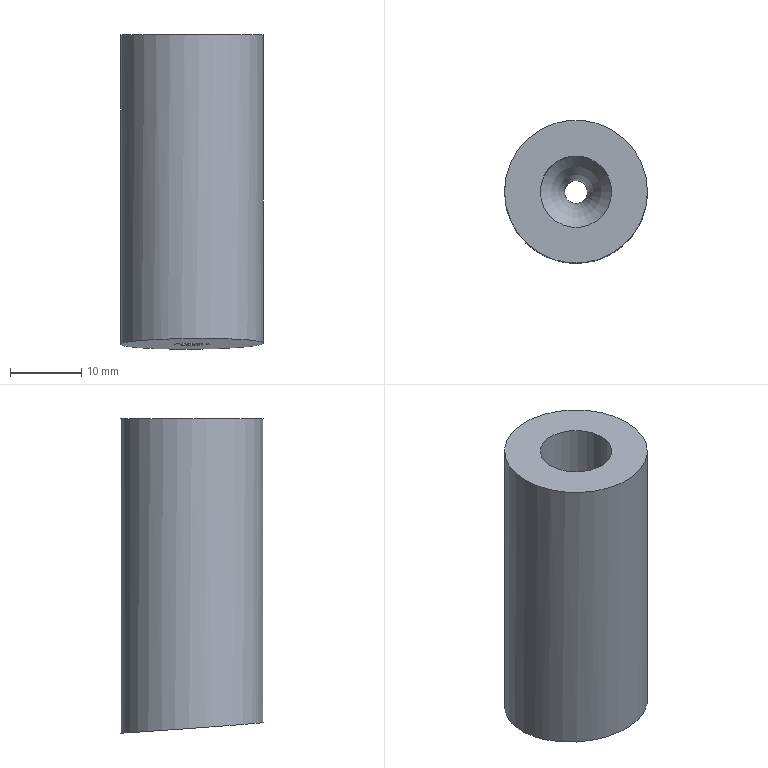Part | NX | features solid 2 | 1 solid | 7 faces | box 20 x 20 x 43.972 mm | volume 10931 mm3 | cylinder 3 | spline 2 | plane 1 | torus 1 | commonest cylinder face diameters 3.2 x1 10 x1 20 x1
STEP:
#1=CARTESIAN_POINT('',(128.211,-387.049,-34.));
#2=VERTEX_POINT('',#1);
#3=CARTESIAN_POINT('',(138.211,-387.049,-34.));
#4=DIRECTION('',(0.,0.,-1.));
#5=DIRECTION('',(-1.,0.,0.));
#6=AXIS2_PLACEMENT_3D('',#3,#4,#5);
#7=CIRCLE('',#6,10.);
#8=EDGE_CURVE('',#2,#2,#7,.T.);
#9=ORIENTED_EDGE('',*,*,#8,.F.);
#10=EDGE_LOOP('',(#9));
#11=FACE_BOUND('',#10,.T.);
#12=CARTESIAN_POINT('',(133.211,-387.049,-34.));
#13=VERTEX_POINT('',#12);
#14=CARTESIAN_POINT('',(138.211,-387.049,-34.));
#15=DIRECTION('',(0.,0.,-1.));
#16=DIRECTION('',(-1.,0.,0.));
#17=AXIS2_PLACEMENT_3D('',#14,#15,#16);
#18=CIRCLE('',#17,5.);
#19=EDGE_CURVE('',#13,#13,#18,.F.);
#20=ORIENTED_EDGE('',*,*,#19,.F.);
#21=EDGE_LOOP('',(#20));
#22=FACE_BOUND('',#21,.T.);
#23=CARTESIAN_POINT('',(138.211,-387.049,-34.));
#24=DIRECTION('',(0.,0.,-1.));
#25=DIRECTION('',(-1.,0.,0.));
#26=AXIS2_PLACEMENT_3D('',#23,#24,#25);
#27=PLANE('',#26);
#28=ADVANCED_FACE('',(#11,#22),#27,.F.);
#29=CARTESIAN_POINT('',(148.211,-387.049,-77.129));
#30=VERTEX_POINT('',#29);
#31=CARTESIAN_POINT('',(146.05,-394.888,-76.557));
#32=CARTESIAN_POINT('',(149.291,-387.046,-77.118));
#33=CARTESIAN_POINT('',(146.054,-379.224,-77.747));
#34=CARTESIAN_POINT('',(138.225,-375.965,-78.053));
#35=CARTESIAN_POINT('',(130.372,-379.213,-77.855));
#36=CARTESIAN_POINT('',(127.134,-387.048,-77.3));
#37=CARTESIAN_POINT('',(130.359,-394.865,-76.71));
#38=CARTESIAN_POINT('',(138.194,-398.136,-76.399));
#39=CARTESIAN_POINT('',(146.05,-394.888,-76.557));
#40=CARTESIAN_POINT('',(149.291,-387.046,-77.118));
#41=CARTESIAN_POINT('',(146.054,-379.224,-77.747));
#42=B_SPLINE_CURVE_WITH_KNOTS('',3,(#31,#32,#33,#34,#35,#36,#37,#38,#39,#40,#41),.UNSPECIFIED.,.T.,.F.,(1,1,1,1,1,1,1,1,1,1,1,1,1,1,1),(-0.02348,-0.01565,-0.007826,0.,0.007826,0.01565,0.02348,0.0313,0.03913,0.04696,0.05478,0.06261,0.07043,0.07826,0.08609),.UNSPECIFIED.);
#43=EDGE_CURVE('',#30,#30,#42,.T.);
#44=ORIENTED_EDGE('',*,*,#43,.T.);
#45=EDGE_LOOP('',(#44));
#46=FACE_BOUND('',#45,.T.);
#47=ORIENTED_EDGE('',*,*,#8,.T.);
#48=EDGE_LOOP('',(#47));
#49=FACE_BOUND('',#48,.T.);
#50=CARTESIAN_POINT('',(138.211,-387.049,-84.));
#51=DIRECTION('',(0.,0.,1.));
#52=DIRECTION('',(1.,0.,0.));
#53=AXIS2_PLACEMENT_3D('',#50,#51,#52);
#54=CYLINDRICAL_SURFACE('',#53,10.);
#55=ADVANCED_FACE('',(#46,#49),#54,.T.);
#56=CARTESIAN_POINT('',(133.211,-387.049,-64.705));
#57=VERTEX_POINT('',#56);
#58=CARTESIAN_POINT('',(138.211,-387.049,-64.705));
#59=DIRECTION('',(0.,0.,-1.));
#60=DIRECTION('',(-1.,0.,0.));
#61=AXIS2_PLACEMENT_3D('',#58,#59,#60);
#62=CIRCLE('',#61,5.);
#63=EDGE_CURVE('',#57,#57,#62,.F.);
#64=ORIENTED_EDGE('',*,*,#63,.F.);
#65=EDGE_LOOP('',(#64));
#66=FACE_BOUND('',#65,.T.);
#67=ORIENTED_EDGE('',*,*,#19,.T.);
#68=EDGE_LOOP('',(#67));
#69=FACE_BOUND('',#68,.T.);
#70=CARTESIAN_POINT('',(138.211,-387.049,-4.));
#71=DIRECTION('',(0.,0.,-1.));
#72=DIRECTION('',(0.,-1.,0.));
#73=AXIS2_PLACEMENT_3D('',#70,#71,#72);
#74=CYLINDRICAL_SURFACE('',#73,5.);
#75=ADVANCED_FACE('',(#66,#69),#74,.F.);
#76=CARTESIAN_POINT('',(138.211,-385.449,-77.354));
#77=VERTEX_POINT('',#76);
#78=CARTESIAN_POINT('',(136.955,-385.798,-77.338));
#79=CARTESIAN_POINT('',(138.212,-385.275,-77.367));
#80=CARTESIAN_POINT('',(139.466,-385.797,-77.318));
#81=CARTESIAN_POINT('',(139.984,-387.047,-77.22));
#82=CARTESIAN_POINT('',(139.468,-388.301,-77.131));
#83=CARTESIAN_POINT('',(138.212,-388.823,-77.103));
#84=CARTESIAN_POINT('',(136.958,-388.303,-77.152));
#85=CARTESIAN_POINT('',(136.439,-387.052,-77.249));
#86=CARTESIAN_POINT('',(136.955,-385.798,-77.338));
#87=CARTESIAN_POINT('',(138.212,-385.275,-77.367));
#88=CARTESIAN_POINT('',(139.466,-385.797,-77.318));
#89=B_SPLINE_CURVE_WITH_KNOTS('',3,(#78,#79,#80,#81,#82,#83,#84,#85,#86,#87,#88),.UNSPECIFIED.,.T.,.F.,(1,1,1,1,1,1,1,1,1,1,1,1,1,1,1),(-0.003757,-0.002504,-0.001252,0.,0.001252,0.002504,0.003757,0.005009,0.006261,0.007513,0.008766,0.01002,0.01127,0.01252,0.01377),.UNSPECIFIED.);
#90=EDGE_CURVE('',#77,#77,#89,.T.);
#91=ORIENTED_EDGE('',*,*,#90,.T.);
#92=EDGE_LOOP('',(#91));
#93=FACE_BOUND('',#92,.T.);
#94=CARTESIAN_POINT('',(139.811,-387.049,-72.614));
#95=VERTEX_POINT('',#94);
#96=CARTESIAN_POINT('',(138.211,-387.049,-72.614));
#97=DIRECTION('',(0.,0.,1.));
#98=DIRECTION('',(1.,0.,0.));
#99=AXIS2_PLACEMENT_3D('',#96,#97,#98);
#100=CIRCLE('',#99,1.6);
#101=EDGE_CURVE('',#95,#95,#100,.F.);
#102=ORIENTED_EDGE('',*,*,#101,.F.);
#103=EDGE_LOOP('',(#102));
#104=FACE_BOUND('',#103,.T.);
#105=CARTESIAN_POINT('',(138.211,-387.049,-94.));
#106=DIRECTION('',(0.,0.,1.));
#107=DIRECTION('',(0.,1.,0.));
#108=AXIS2_PLACEMENT_3D('',#105,#106,#107);
#109=CYLINDRICAL_SURFACE('',#108,1.6);
#110=ADVANCED_FACE('',(#93,#104),#109,.F.);
#111=ORIENTED_EDGE('',*,*,#101,.T.);
#112=EDGE_LOOP('',(#111));
#113=FACE_BOUND('',#112,.T.);
#114=ORIENTED_EDGE('',*,*,#63,.T.);
#115=EDGE_LOOP('',(#114));
#116=FACE_BOUND('',#115,.T.);
#117=CARTESIAN_POINT('',(138.211,-387.049,-72.614));
#118=DIRECTION('',(0.,0.,1.));
#119=DIRECTION('',(1.,0.,0.));
#120=AXIS2_PLACEMENT_3D('',#117,#118,#119);
#121=TOROIDAL_SURFACE('',#120,12.5,10.9);
#122=ADVANCED_FACE('',(#113,#116),#121,.T.);
#123=CARTESIAN_POINT('',(139.227,-384.777,-77.396));
#124=VERTEX_POINT('',#123);
#125=CARTESIAN_POINT('',(137.177,-389.327,-77.073));
#126=VERTEX_POINT('',#125);
#127=CARTESIAN_POINT('',(139.227,-384.777,-77.396));
#128=CARTESIAN_POINT('',(139.852,-385.057,-77.37));
#129=CARTESIAN_POINT('',(140.767,-386.043,-77.288));
#130=CARTESIAN_POINT('',(140.747,-388.181,-77.128));
#131=CARTESIAN_POINT('',(139.156,-389.633,-77.034));
#132=CARTESIAN_POINT('',(137.804,-389.608,-77.047));
#133=CARTESIAN_POINT('',(137.177,-389.327,-77.073));
#134=B_SPLINE_CURVE_WITH_KNOTS('',3,(#127,#128,#129,#130,#131,#132,#133),.UNSPECIFIED.,.F.,.F.,(4,1,1,1,4),(0.,0.25,0.5,0.75,1.),.UNSPECIFIED.);
#135=EDGE_CURVE('',#124,#126,#134,.T.);
#136=ORIENTED_EDGE('',*,*,#135,.F.);
#137=CARTESIAN_POINT('',(137.177,-389.327,-77.073));
#138=CARTESIAN_POINT('',(136.552,-389.047,-77.099));
#139=CARTESIAN_POINT('',(135.638,-388.06,-77.18));
#140=CARTESIAN_POINT('',(135.657,-385.922,-77.338));
#141=CARTESIAN_POINT('',(137.248,-384.471,-77.434));
#142=CARTESIAN_POINT('',(138.6,-384.497,-77.422));
#143=CARTESIAN_POINT('',(139.227,-384.777,-77.396));
#144=B_SPLINE_CURVE_WITH_KNOTS('',3,(#137,#138,#139,#140,#141,#142,#143),.UNSPECIFIED.,.F.,.F.,(4,1,1,1,4),(0.,0.25,0.5,0.75,1.),.UNSPECIFIED.);
#145=EDGE_CURVE('',#126,#124,#144,.T.);
#146=ORIENTED_EDGE('',*,*,#145,.F.);
#147=EDGE_LOOP('',(#136,#146));
#148=FACE_BOUND('',#147,.T.);
#149=ORIENTED_EDGE('',*,*,#43,.F.);
#150=EDGE_LOOP('',(#149));
#151=FACE_BOUND('',#150,.T.);
#152=CARTESIAN_POINT('',(148.264,-397.014,-76.359));
#153=CARTESIAN_POINT('',(144.203,-397.08,-76.412));
#154=CARTESIAN_POINT('',(140.141,-397.144,-76.456));
#155=CARTESIAN_POINT('',(136.08,-397.206,-76.49));
#156=CARTESIAN_POINT('',(132.018,-397.265,-76.515));
#157=CARTESIAN_POINT('',(127.955,-397.323,-76.531));
#158=CARTESIAN_POINT('',(148.294,-392.955,-76.677));
#159=CARTESIAN_POINT('',(144.233,-393.02,-76.728));
#160=CARTESIAN_POINT('',(140.171,-393.083,-76.77));
#161=CARTESIAN_POINT('',(136.109,-393.144,-76.802));
#162=CARTESIAN_POINT('',(132.047,-393.202,-76.824));
#163=CARTESIAN_POINT('',(127.985,-393.259,-76.838));
#164=CARTESIAN_POINT('',(148.324,-388.896,-76.99));
#165=CARTESIAN_POINT('',(144.263,-388.96,-77.039));
#166=CARTESIAN_POINT('',(140.201,-389.022,-77.079));
#167=CARTESIAN_POINT('',(136.139,-389.082,-77.108));
#168=CARTESIAN_POINT('',(132.077,-389.14,-77.129));
#169=CARTESIAN_POINT('',(128.014,-389.195,-77.14));
#170=CARTESIAN_POINT('',(148.353,-384.836,-77.298));
#171=CARTESIAN_POINT('',(144.292,-384.899,-77.345));
#172=CARTESIAN_POINT('',(140.23,-384.961,-77.382));
#173=CARTESIAN_POINT('',(136.168,-385.02,-77.41));
#174=CARTESIAN_POINT('',(132.105,-385.076,-77.428));
#175=CARTESIAN_POINT('',(128.043,-385.131,-77.437));
#176=CARTESIAN_POINT('',(148.382,-380.777,-77.601));
#177=CARTESIAN_POINT('',(144.32,-380.839,-77.646));
#178=CARTESIAN_POINT('',(140.259,-380.899,-77.681));
#179=CARTESIAN_POINT('',(136.196,-380.957,-77.707));
#180=CARTESIAN_POINT('',(132.134,-381.013,-77.723));
#181=CARTESIAN_POINT('',(128.071,-381.067,-77.73));
#182=CARTESIAN_POINT('',(148.41,-376.717,-77.899));
#183=CARTESIAN_POINT('',(144.349,-376.778,-77.942));
#184=CARTESIAN_POINT('',(140.287,-376.838,-77.975));
#185=CARTESIAN_POINT('',(136.224,-376.895,-77.998));
#186=CARTESIAN_POINT('',(132.162,-376.95,-78.012));
#187=CARTESIAN_POINT('',(128.099,-377.003,-78.017));
#188=B_SPLINE_SURFACE_WITH_KNOTS('',5,5,((#152,#153,#154,#155,#156,#157),(#158,#159,#160,#161,#162,#163),(#164,#165,#166,#167,#168,#169),(#170,#171,#172,#173,#174,#175),(#176,#177,#178,#179,#180,#181),(#182,#183,#184,#185,#186,#187)),.UNSPECIFIED.,.F.,.F.,.F.,(6,6),(6,6),(0.3021,0.7045),(0.1174,0.8783),.PIECEWISE_BEZIER_KNOTS.);
#189=ADVANCED_FACE('',(#148,#151),#188,.F.);
#190=ORIENTED_EDGE('',*,*,#145,.T.);
#191=ORIENTED_EDGE('',*,*,#135,.T.);
#192=EDGE_LOOP('',(#190,#191));
#193=FACE_BOUND('',#192,.T.);
#194=ORIENTED_EDGE('',*,*,#90,.F.);
#195=EDGE_LOOP('',(#194));
#196=FACE_BOUND('',#195,.T.);
#197=CARTESIAN_POINT('',(140.732,-389.566,-77.024));
#198=CARTESIAN_POINT('',(139.675,-389.582,-77.033));
#199=CARTESIAN_POINT('',(138.617,-389.597,-77.041));
#200=CARTESIAN_POINT('',(137.56,-389.613,-77.049));
#201=CARTESIAN_POINT('',(136.502,-389.629,-77.056));
#202=CARTESIAN_POINT('',(135.445,-389.644,-77.063));
#203=CARTESIAN_POINT('',(140.74,-388.51,-77.103));
#204=CARTESIAN_POINT('',(139.682,-388.526,-77.112));
#205=CARTESIAN_POINT('',(138.625,-388.542,-77.121));
#206=CARTESIAN_POINT('',(137.568,-388.557,-77.128));
#207=CARTESIAN_POINT('',(136.51,-388.573,-77.135));
#208=CARTESIAN_POINT('',(135.453,-388.588,-77.142));
#209=CARTESIAN_POINT('',(140.747,-387.455,-77.183));
#210=CARTESIAN_POINT('',(139.69,-387.471,-77.191));
#211=CARTESIAN_POINT('',(138.633,-387.486,-77.2));
#212=CARTESIAN_POINT('',(137.575,-387.502,-77.207));
#213=CARTESIAN_POINT('',(136.518,-387.517,-77.214));
#214=CARTESIAN_POINT('',(135.46,-387.532,-77.22));
#215=CARTESIAN_POINT('',(140.755,-386.399,-77.262));
#216=CARTESIAN_POINT('',(139.698,-386.415,-77.27));
#217=CARTESIAN_POINT('',(138.64,-386.431,-77.278));
#218=CARTESIAN_POINT('',(137.583,-386.446,-77.286));
#219=CARTESIAN_POINT('',(136.525,-386.461,-77.292));
#220=CARTESIAN_POINT('',(135.468,-386.477,-77.299));
#221=CARTESIAN_POINT('',(140.763,-385.344,-77.34));
#222=CARTESIAN_POINT('',(139.705,-385.36,-77.349));
#223=CARTESIAN_POINT('',(138.648,-385.375,-77.357));
#224=CARTESIAN_POINT('',(137.59,-385.391,-77.364));
#225=CARTESIAN_POINT('',(136.533,-385.406,-77.371));
#226=CARTESIAN_POINT('',(135.475,-385.421,-77.376));
#227=CARTESIAN_POINT('',(140.77,-384.289,-77.419));
#228=CARTESIAN_POINT('',(139.713,-384.304,-77.427));
#229=CARTESIAN_POINT('',(138.655,-384.32,-77.435));
#230=CARTESIAN_POINT('',(137.598,-384.335,-77.442));
#231=CARTESIAN_POINT('',(136.54,-384.35,-77.448));
#232=CARTESIAN_POINT('',(135.483,-384.365,-77.454));
#233=B_SPLINE_SURFACE_WITH_KNOTS('',5,5,((#197,#198,#199,#200,#201,#202),(#203,#204,#205,#206,#207,#208),(#209,#210,#211,#212,#213,#214),(#215,#216,#217,#218,#219,#220),(#221,#222,#223,#224,#225,#226),(#227,#228,#229,#230,#231,#232)),.UNSPECIFIED.,.F.,.F.,.F.,(6,6),(6,6),(0.4521,0.5567),(0.4017,0.5997),.PIECEWISE_BEZIER_KNOTS.);
#234=ADVANCED_FACE('',(#193,#196),#233,.F.);
#235=CLOSED_SHELL('',(#28,#55,#75,#110,#122,#189,#234));
#236=MANIFOLD_SOLID_BREP('',#235);
#237=(LENGTH_UNIT()NAMED_UNIT(*)SI_UNIT(.MILLI.,.METRE.));
#238=UNCERTAINTY_MEASURE_WITH_UNIT(LENGTH_MEASURE(0.0508),#237,'','');
#239=(NAMED_UNIT(*)PLANE_ANGLE_UNIT()SI_UNIT($,.RADIAN.));
#240=(NAMED_UNIT(*)SI_UNIT($,.STERADIAN.)SOLID_ANGLE_UNIT());
#241=(GEOMETRIC_REPRESENTATION_CONTEXT(3)GLOBAL_UNCERTAINTY_ASSIGNED_CONTEXT((#238))GLOBAL_UNIT_ASSIGNED_CONTEXT((#237,#239,#240))REPRESENTATION_CONTEXT('',''));
#242=ADVANCED_BREP_SHAPE_REPRESENTATION('',(#236),#241);